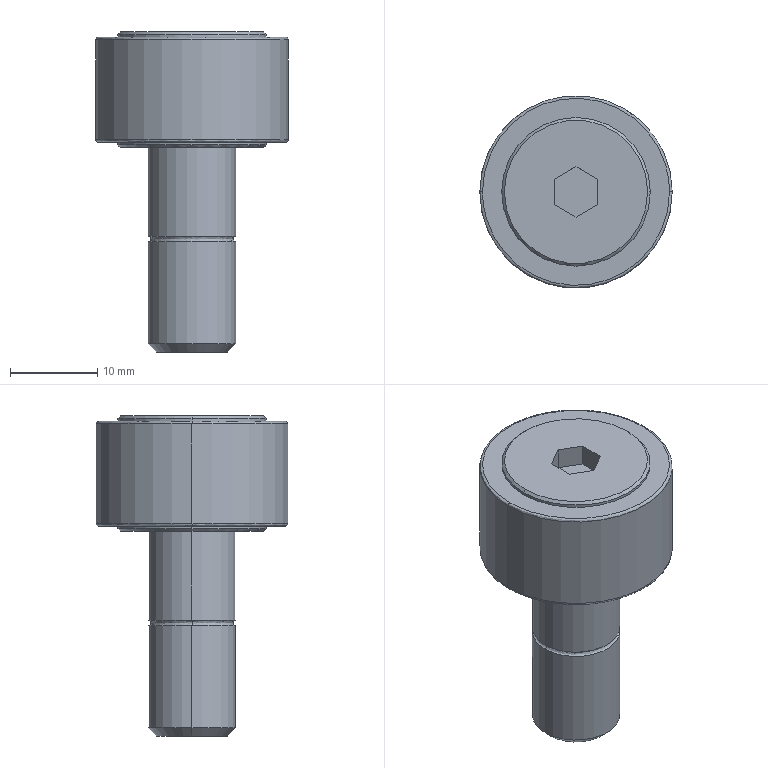Part | SolidWorks | features BaseBody 2 | 1 solid | 41 faces | box 22 x 22 x 36.6 mm | volume 6559 mm3 | plane 13 | cylinder 12 | cone 10 | spline 6 | commonest cylinder face diameters 10 x4 17 x4 3.242 x2 22 x2
STEP:
#1=CARTESIAN_POINT('',(11.,0.,-0.9));
#2=VERTEX_POINT('',#1);
#3=CARTESIAN_POINT('',(-11.,0.,-0.9));
#4=VERTEX_POINT('',#3);
#5=CARTESIAN_POINT('',(0.,0.,-0.9));
#6=DIRECTION('',(0.,0.,-1.));
#7=DIRECTION('',(1.,0.,0.));
#8=AXIS2_PLACEMENT_3D('',#5,#6,#7);
#9=CIRCLE('',#8,11.);
#10=EDGE_CURVE('',#2,#4,#9,.T.);
#11=ORIENTED_EDGE('',*,*,#10,.F.);
#12=CARTESIAN_POINT('',(10.7,0.,-0.6));
#13=VERTEX_POINT('',#12);
#14=CARTESIAN_POINT('',(10.7,0.,-0.9));
#15=DIRECTION('',(0.,-1.,0.));
#16=DIRECTION('',(1.,0.,0.));
#17=AXIS2_PLACEMENT_3D('',#14,#15,#16);
#18=CIRCLE('',#17,0.3);
#19=EDGE_CURVE('',#2,#13,#18,.T.);
#20=ORIENTED_EDGE('',*,*,#19,.T.);
#21=CARTESIAN_POINT('',(-10.7,0.,-0.6));
#22=VERTEX_POINT('',#21);
#23=CARTESIAN_POINT('',(10.7,0.,-0.6));
#24=CARTESIAN_POINT('',(10.7,-21.4,-0.6));
#25=CARTESIAN_POINT('',(-10.7,-21.4,-0.6));
#26=CARTESIAN_POINT('',(-10.7,0.,-0.6));
#27=(BOUNDED_CURVE()B_SPLINE_CURVE(3,(#23,#24,#25,#26),.UNSPECIFIED.,.F.,.T.)B_SPLINE_CURVE_WITH_KNOTS((4,4),(0.5,1.),.UNSPECIFIED.)CURVE()GEOMETRIC_REPRESENTATION_ITEM()RATIONAL_B_SPLINE_CURVE((1.,0.3333,0.3333,1.))REPRESENTATION_ITEM(''));
#28=EDGE_CURVE('',#13,#22,#27,.T.);
#29=ORIENTED_EDGE('',*,*,#28,.T.);
#30=CARTESIAN_POINT('',(-10.7,0.,-0.9));
#31=DIRECTION('',(0.,1.,0.));
#32=DIRECTION('',(-1.,0.,0.));
#33=AXIS2_PLACEMENT_3D('',#30,#31,#32);
#34=CIRCLE('',#33,0.3);
#35=EDGE_CURVE('',#4,#22,#34,.T.);
#36=ORIENTED_EDGE('',*,*,#35,.F.);
#37=EDGE_LOOP('',(#11,#20,#29,#36));
#38=FACE_OUTER_BOUND('',#37,.T.);
#39=CARTESIAN_POINT('',(11.,0.,-0.9));
#40=CARTESIAN_POINT('',(11.,-22.,-0.9));
#41=CARTESIAN_POINT('',(-11.,-22.,-0.9));
#42=CARTESIAN_POINT('',(-11.,0.,-0.9));
#43=CARTESIAN_POINT('',(11.,0.,-0.7243));
#44=CARTESIAN_POINT('',(11.,-22.,-0.7243));
#45=CARTESIAN_POINT('',(-11.,-22.,-0.7243));
#46=CARTESIAN_POINT('',(-11.,0.,-0.7243));
#47=CARTESIAN_POINT('',(10.876,0.,-0.6));
#48=CARTESIAN_POINT('',(10.876,-21.751,-0.6));
#49=CARTESIAN_POINT('',(-10.876,-21.751,-0.6));
#50=CARTESIAN_POINT('',(-10.876,0.,-0.6));
#51=CARTESIAN_POINT('',(10.7,0.,-0.6));
#52=CARTESIAN_POINT('',(10.7,-21.4,-0.6));
#53=CARTESIAN_POINT('',(-10.7,-21.4,-0.6));
#54=CARTESIAN_POINT('',(-10.7,0.,-0.6));
#55=(BOUNDED_SURFACE()B_SPLINE_SURFACE(3,3,((#39,#40,#41,#42),(#43,#44,#45,#46),(#47,#48,#49,#50),(#51,#52,#53,#54)),.UNSPECIFIED.,.F.,.F.,.T.)B_SPLINE_SURFACE_WITH_KNOTS((4,4),(4,4),(0.,1.),(0.,1.),.UNSPECIFIED.)GEOMETRIC_REPRESENTATION_ITEM()RATIONAL_B_SPLINE_SURFACE(((1.,0.3333,0.3333,1.),(0.8047,0.2682,0.2682,0.8047),(0.8047,0.2682,0.2682,0.8047),(1.,0.3333,0.3333,1.)))REPRESENTATION_ITEM('')SURFACE());
#56=ADVANCED_FACE('',(#38),#55,.T.);
#57=CARTESIAN_POINT('',(-10.7,0.,-12.6));
#58=VERTEX_POINT('',#57);
#59=CARTESIAN_POINT('',(10.7,0.,-12.6));
#60=VERTEX_POINT('',#59);
#61=CARTESIAN_POINT('',(-10.7,0.,-12.6));
#62=CARTESIAN_POINT('',(-10.7,-21.4,-12.6));
#63=CARTESIAN_POINT('',(10.7,-21.4,-12.6));
#64=CARTESIAN_POINT('',(10.7,0.,-12.6));
#65=(BOUNDED_CURVE()B_SPLINE_CURVE(3,(#61,#62,#63,#64),.UNSPECIFIED.,.F.,.T.)B_SPLINE_CURVE_WITH_KNOTS((4,4),(0.,0.5),.UNSPECIFIED.)CURVE()GEOMETRIC_REPRESENTATION_ITEM()RATIONAL_B_SPLINE_CURVE((1.,0.3333,0.3333,1.))REPRESENTATION_ITEM(''));
#66=EDGE_CURVE('',#58,#60,#65,.T.);
#67=ORIENTED_EDGE('',*,*,#66,.T.);
#68=CARTESIAN_POINT('',(11.,0.,-12.3));
#69=VERTEX_POINT('',#68);
#70=CARTESIAN_POINT('',(10.7,0.,-12.3));
#71=DIRECTION('',(0.,-1.,0.));
#72=DIRECTION('',(1.,0.,0.));
#73=AXIS2_PLACEMENT_3D('',#70,#71,#72);
#74=CIRCLE('',#73,0.3);
#75=EDGE_CURVE('',#60,#69,#74,.T.);
#76=ORIENTED_EDGE('',*,*,#75,.T.);
#77=CARTESIAN_POINT('',(-11.,0.,-12.3));
#78=VERTEX_POINT('',#77);
#79=CARTESIAN_POINT('',(0.,0.,-12.3));
#80=DIRECTION('',(0.,0.,1.));
#81=DIRECTION('',(1.,0.,0.));
#82=AXIS2_PLACEMENT_3D('',#79,#80,#81);
#83=CIRCLE('',#82,11.);
#84=EDGE_CURVE('',#78,#69,#83,.T.);
#85=ORIENTED_EDGE('',*,*,#84,.F.);
#86=CARTESIAN_POINT('',(-10.7,0.,-12.3));
#87=DIRECTION('',(0.,1.,0.));
#88=DIRECTION('',(-1.,0.,0.));
#89=AXIS2_PLACEMENT_3D('',#86,#87,#88);
#90=CIRCLE('',#89,0.3);
#91=EDGE_CURVE('',#58,#78,#90,.T.);
#92=ORIENTED_EDGE('',*,*,#91,.F.);
#93=EDGE_LOOP('',(#67,#76,#85,#92));
#94=FACE_OUTER_BOUND('',#93,.T.);
#95=CARTESIAN_POINT('',(10.7,0.,-12.6));
#96=CARTESIAN_POINT('',(10.7,-21.4,-12.6));
#97=CARTESIAN_POINT('',(-10.7,-21.4,-12.6));
#98=CARTESIAN_POINT('',(-10.7,0.,-12.6));
#99=CARTESIAN_POINT('',(10.876,0.,-12.6));
#100=CARTESIAN_POINT('',(10.876,-21.751,-12.6));
#101=CARTESIAN_POINT('',(-10.876,-21.751,-12.6));
#102=CARTESIAN_POINT('',(-10.876,0.,-12.6));
#103=CARTESIAN_POINT('',(11.,0.,-12.476));
#104=CARTESIAN_POINT('',(11.,-22.,-12.476));
#105=CARTESIAN_POINT('',(-11.,-22.,-12.476));
#106=CARTESIAN_POINT('',(-11.,0.,-12.476));
#107=CARTESIAN_POINT('',(11.,0.,-12.3));
#108=CARTESIAN_POINT('',(11.,-22.,-12.3));
#109=CARTESIAN_POINT('',(-11.,-22.,-12.3));
#110=CARTESIAN_POINT('',(-11.,0.,-12.3));
#111=(BOUNDED_SURFACE()B_SPLINE_SURFACE(3,3,((#95,#96,#97,#98),(#99,#100,#101,#102),(#103,#104,#105,#106),(#107,#108,#109,#110)),.UNSPECIFIED.,.F.,.F.,.F.)B_SPLINE_SURFACE_WITH_KNOTS((4,4),(4,4),(0.,1.),(0.,1.),.UNSPECIFIED.)GEOMETRIC_REPRESENTATION_ITEM()RATIONAL_B_SPLINE_SURFACE(((1.,0.3333,0.3333,1.),(0.8047,0.2682,0.2682,0.8047),(0.8047,0.2682,0.2682,0.8047),(1.,0.3333,0.3333,1.)))REPRESENTATION_ITEM('')SURFACE());
#112=ADVANCED_FACE('',(#94),#111,.T.);
#113=CARTESIAN_POINT('',(5.,0.,-23.375));
#114=VERTEX_POINT('',#113);
#115=CARTESIAN_POINT('',(-5.,0.,-23.375));
#116=VERTEX_POINT('',#115);
#117=CARTESIAN_POINT('',(0.,0.,-23.375));
#118=DIRECTION('',(0.,0.,1.));
#119=DIRECTION('',(1.,0.,0.));
#120=AXIS2_PLACEMENT_3D('',#117,#118,#119);
#121=CIRCLE('',#120,5.);
#122=EDGE_CURVE('',#114,#116,#121,.T.);
#123=ORIENTED_EDGE('',*,*,#122,.F.);
#124=CARTESIAN_POINT('',(5.,0.,-23.975));
#125=VERTEX_POINT('',#124);
#126=CARTESIAN_POINT('',(5.,0.,-23.675));
#127=DIRECTION('',(0.,-1.,0.));
#128=DIRECTION('',(1.,0.,0.));
#129=AXIS2_PLACEMENT_3D('',#126,#127,#128);
#130=CIRCLE('',#129,0.3);
#131=EDGE_CURVE('',#114,#125,#130,.T.);
#132=ORIENTED_EDGE('',*,*,#131,.T.);
#133=CARTESIAN_POINT('',(-5.,0.,-23.975));
#134=VERTEX_POINT('',#133);
#135=CARTESIAN_POINT('',(0.,0.,-23.975));
#136=DIRECTION('',(0.,0.,-1.));
#137=DIRECTION('',(-1.,0.,0.));
#138=AXIS2_PLACEMENT_3D('',#135,#136,#137);
#139=CIRCLE('',#138,5.);
#140=EDGE_CURVE('',#134,#125,#139,.T.);
#141=ORIENTED_EDGE('',*,*,#140,.F.);
#142=CARTESIAN_POINT('',(-5.,0.,-23.675));
#143=DIRECTION('',(0.,1.,0.));
#144=DIRECTION('',(-1.,0.,0.));
#145=AXIS2_PLACEMENT_3D('',#142,#143,#144);
#146=CIRCLE('',#145,0.3);
#147=EDGE_CURVE('',#116,#134,#146,.T.);
#148=ORIENTED_EDGE('',*,*,#147,.F.);
#149=EDGE_LOOP('',(#123,#132,#141,#148));
#150=FACE_OUTER_BOUND('',#149,.T.);
#151=CARTESIAN_POINT('',(-5.,0.,-23.375));
#152=CARTESIAN_POINT('',(-5.,10.,-23.375));
#153=CARTESIAN_POINT('',(5.,10.,-23.375));
#154=CARTESIAN_POINT('',(5.,0.,-23.375));
#155=CARTESIAN_POINT('',(-4.4,0.,-23.375));
#156=CARTESIAN_POINT('',(-4.4,8.8,-23.375));
#157=CARTESIAN_POINT('',(4.4,8.8,-23.375));
#158=CARTESIAN_POINT('',(4.4,0.,-23.375));
#159=CARTESIAN_POINT('',(-4.4,0.,-23.975));
#160=CARTESIAN_POINT('',(-4.4,8.8,-23.975));
#161=CARTESIAN_POINT('',(4.4,8.8,-23.975));
#162=CARTESIAN_POINT('',(4.4,0.,-23.975));
#163=CARTESIAN_POINT('',(-5.,0.,-23.975));
#164=CARTESIAN_POINT('',(-5.,10.,-23.975));
#165=CARTESIAN_POINT('',(5.,10.,-23.975));
#166=CARTESIAN_POINT('',(5.,0.,-23.975));
#167=(BOUNDED_SURFACE()B_SPLINE_SURFACE(3,3,((#151,#152,#153,#154),(#155,#156,#157,#158),(#159,#160,#161,#162),(#163,#164,#165,#166)),.UNSPECIFIED.,.F.,.F.,.F.)B_SPLINE_SURFACE_WITH_KNOTS((4,4),(4,4),(0.,1.),(0.,1.),.UNSPECIFIED.)GEOMETRIC_REPRESENTATION_ITEM()RATIONAL_B_SPLINE_SURFACE(((1.,0.3333,0.3333,1.),(0.3333,0.1111,0.1111,0.3333),(0.3333,0.1111,0.1111,0.3333),(1.,0.3333,0.3333,1.)))REPRESENTATION_ITEM('')SURFACE());
#168=ADVANCED_FACE('',(#150),#167,.F.);
#169=CARTESIAN_POINT('',(0.,0.,-12.3));
#170=DIRECTION('',(0.,0.,1.));
#171=DIRECTION('',(1.,0.,0.));
#172=AXIS2_PLACEMENT_3D('',#169,#170,#171);
#173=CIRCLE('',#172,11.);
#174=EDGE_CURVE('',#69,#78,#173,.T.);
#175=ORIENTED_EDGE('',*,*,#174,.T.);
#176=CARTESIAN_POINT('',(-11.,0.,-36.6));
#177=DIRECTION('',(0.,0.,1.));
#178=VECTOR('',#177,1000.);
#179=LINE('',#176,#178);
#180=EDGE_CURVE('',#78,#4,#179,.T.);
#181=ORIENTED_EDGE('',*,*,#180,.T.);
#182=CARTESIAN_POINT('',(0.,0.,-0.9));
#183=DIRECTION('',(0.,0.,-1.));
#184=DIRECTION('',(1.,0.,0.));
#185=AXIS2_PLACEMENT_3D('',#182,#183,#184);
#186=CIRCLE('',#185,11.);
#187=EDGE_CURVE('',#4,#2,#186,.T.);
#188=ORIENTED_EDGE('',*,*,#187,.T.);
#189=CARTESIAN_POINT('',(11.,0.,-36.6));
#190=DIRECTION('',(0.,0.,1.));
#191=VECTOR('',#190,1000.);
#192=LINE('',#189,#191);
#193=EDGE_CURVE('',#69,#2,#192,.T.);
#194=ORIENTED_EDGE('',*,*,#193,.F.);
#195=EDGE_LOOP('',(#175,#181,#188,#194));
#196=FACE_OUTER_BOUND('',#195,.T.);
#197=CARTESIAN_POINT('',(0.,0.,-36.6));
#198=DIRECTION('',(0.,0.,1.));
#199=DIRECTION('',(1.,0.,0.));
#200=AXIS2_PLACEMENT_3D('',#197,#198,#199);
#201=CYLINDRICAL_SURFACE('',#200,11.);
#202=ADVANCED_FACE('',(#196),#201,.T.);
#203=CARTESIAN_POINT('',(8.5,0.,-0.6));
#204=VERTEX_POINT('',#203);
#205=CARTESIAN_POINT('',(-8.5,0.,-0.6));
#206=VERTEX_POINT('',#205);
#207=CARTESIAN_POINT('',(0.,0.,-0.6));
#208=DIRECTION('',(0.,0.,1.));
#209=DIRECTION('',(1.,0.,0.));
#210=AXIS2_PLACEMENT_3D('',#207,#208,#209);
#211=CIRCLE('',#210,8.5);
#212=EDGE_CURVE('',#204,#206,#211,.T.);
#213=ORIENTED_EDGE('',*,*,#212,.T.);
#214=CARTESIAN_POINT('',(-8.5,0.,-0.3));
#215=VERTEX_POINT('',#214);
#216=CARTESIAN_POINT('',(-8.5,0.,-36.6));
#217=DIRECTION('',(0.,0.,1.));
#218=VECTOR('',#217,1000.);
#219=LINE('',#216,#218);
#220=EDGE_CURVE('',#206,#215,#219,.T.);
#221=ORIENTED_EDGE('',*,*,#220,.T.);
#222=CARTESIAN_POINT('',(8.5,0.,-0.3));
#223=VERTEX_POINT('',#222);
#224=CARTESIAN_POINT('',(0.,0.,-0.3));
#225=DIRECTION('',(0.,0.,-1.));
#226=DIRECTION('',(1.,0.,0.));
#227=AXIS2_PLACEMENT_3D('',#224,#225,#226);
#228=CIRCLE('',#227,8.5);
#229=EDGE_CURVE('',#215,#223,#228,.T.);
#230=ORIENTED_EDGE('',*,*,#229,.T.);
#231=CARTESIAN_POINT('',(8.5,0.,-36.6));
#232=DIRECTION('',(0.,0.,1.));
#233=VECTOR('',#232,1000.);
#234=LINE('',#231,#233);
#235=EDGE_CURVE('',#204,#223,#234,.T.);
#236=ORIENTED_EDGE('',*,*,#235,.F.);
#237=EDGE_LOOP('',(#213,#221,#230,#236));
#238=FACE_OUTER_BOUND('',#237,.T.);
#239=CARTESIAN_POINT('',(0.,0.,-36.6));
#240=DIRECTION('',(0.,0.,1.));
#241=DIRECTION('',(1.,0.,0.));
#242=AXIS2_PLACEMENT_3D('',#239,#240,#241);
#243=CYLINDRICAL_SURFACE('',#242,8.5);
#244=ADVANCED_FACE('',(#238),#243,.T.);
#245=CARTESIAN_POINT('',(8.5,0.,-12.9));
#246=VERTEX_POINT('',#245);
#247=CARTESIAN_POINT('',(-8.5,0.,-12.9));
#248=VERTEX_POINT('',#247);
#249=CARTESIAN_POINT('',(0.,0.,-12.9));
#250=DIRECTION('',(0.,0.,1.));
#251=DIRECTION('',(1.,0.,0.));
#252=AXIS2_PLACEMENT_3D('',#249,#250,#251);
#253=CIRCLE('',#252,8.5);
#254=EDGE_CURVE('',#246,#248,#253,.T.);
#255=ORIENTED_EDGE('',*,*,#254,.T.);
#256=CARTESIAN_POINT('',(-8.5,0.,-12.6));
#257=VERTEX_POINT('',#256);
#258=CARTESIAN_POINT('',(-8.5,0.,-36.6));
#259=DIRECTION('',(0.,0.,1.));
#260=VECTOR('',#259,1000.);
#261=LINE('',#258,#260);
#262=EDGE_CURVE('',#248,#257,#261,.T.);
#263=ORIENTED_EDGE('',*,*,#262,.T.);
#264=CARTESIAN_POINT('',(8.5,0.,-12.6));
#265=VERTEX_POINT('',#264);
#266=CARTESIAN_POINT('',(0.,0.,-12.6));
#267=DIRECTION('',(0.,0.,-1.));
#268=DIRECTION('',(1.,0.,0.));
#269=AXIS2_PLACEMENT_3D('',#266,#267,#268);
#270=CIRCLE('',#269,8.5);
#271=EDGE_CURVE('',#257,#265,#270,.T.);
#272=ORIENTED_EDGE('',*,*,#271,.T.);
#273=CARTESIAN_POINT('',(8.5,0.,-36.6));
#274=DIRECTION('',(0.,0.,1.));
#275=VECTOR('',#274,1000.);
#276=LINE('',#273,#275);
#277=EDGE_CURVE('',#246,#265,#276,.T.);
#278=ORIENTED_EDGE('',*,*,#277,.F.);
#279=EDGE_LOOP('',(#255,#263,#272,#278));
#280=FACE_OUTER_BOUND('',#279,.T.);
#281=CARTESIAN_POINT('',(0.,0.,-36.6));
#282=DIRECTION('',(0.,0.,1.));
#283=DIRECTION('',(1.,0.,0.));
#284=AXIS2_PLACEMENT_3D('',#281,#282,#283);
#285=CYLINDRICAL_SURFACE('',#284,8.5);
#286=ADVANCED_FACE('',(#280),#285,.T.);
#287=CARTESIAN_POINT('',(-8.2,0.,0.));
#288=VERTEX_POINT('',#287);
#289=CARTESIAN_POINT('',(8.2,0.,0.));
#290=VERTEX_POINT('',#289);
#291=CARTESIAN_POINT('',(0.,0.,0.));
#292=DIRECTION('',(0.,0.,-1.));
#293=DIRECTION('',(-1.,0.,0.));
#294=AXIS2_PLACEMENT_3D('',#291,#292,#293);
#295=CIRCLE('',#294,8.2);
#296=EDGE_CURVE('',#288,#290,#295,.T.);
#297=ORIENTED_EDGE('',*,*,#296,.T.);
#298=CARTESIAN_POINT('',(8.5,0.,-0.3));
#299=DIRECTION('',(0.7071,0.,-0.7071));
#300=VECTOR('',#299,1000.);
#301=LINE('',#298,#300);
#302=EDGE_CURVE('',#290,#223,#301,.T.);
#303=ORIENTED_EDGE('',*,*,#302,.T.);
#304=ORIENTED_EDGE('',*,*,#229,.F.);
#305=CARTESIAN_POINT('',(-8.5,0.,-0.3));
#306=DIRECTION('',(-0.7071,0.,-0.7071));
#307=VECTOR('',#306,1000.);
#308=LINE('',#305,#307);
#309=EDGE_CURVE('',#288,#215,#308,.T.);
#310=ORIENTED_EDGE('',*,*,#309,.F.);
#311=EDGE_LOOP('',(#297,#303,#304,#310));
#312=FACE_OUTER_BOUND('',#311,.T.);
#313=CARTESIAN_POINT('',(0.,0.,-0.3));
#314=DIRECTION('',(0.,0.,-1.));
#315=DIRECTION('',(-1.,0.,0.));
#316=AXIS2_PLACEMENT_3D('',#313,#314,#315);
#317=CONICAL_SURFACE('',#316,8.5,0.7854);
#318=ADVANCED_FACE('',(#312),#317,.T.);
#319=CARTESIAN_POINT('',(8.2,0.,-13.2));
#320=VERTEX_POINT('',#319);
#321=CARTESIAN_POINT('',(-8.2,0.,-13.2));
#322=VERTEX_POINT('',#321);
#323=CARTESIAN_POINT('',(0.,0.,-13.2));
#324=DIRECTION('',(0.,0.,1.));
#325=DIRECTION('',(1.,0.,0.));
#326=AXIS2_PLACEMENT_3D('',#323,#324,#325);
#327=CIRCLE('',#326,8.2);
#328=EDGE_CURVE('',#320,#322,#327,.T.);
#329=ORIENTED_EDGE('',*,*,#328,.T.);
#330=CARTESIAN_POINT('',(-8.5,0.,-12.9));
#331=DIRECTION('',(-0.7071,0.,0.7071));
#332=VECTOR('',#331,1000.);
#333=LINE('',#330,#332);
#334=EDGE_CURVE('',#322,#248,#333,.T.);
#335=ORIENTED_EDGE('',*,*,#334,.T.);
#336=ORIENTED_EDGE('',*,*,#254,.F.);
#337=CARTESIAN_POINT('',(8.5,0.,-12.9));
#338=DIRECTION('',(0.7071,0.,0.7071));
#339=VECTOR('',#338,1000.);
#340=LINE('',#337,#339);
#341=EDGE_CURVE('',#320,#246,#340,.T.);
#342=ORIENTED_EDGE('',*,*,#341,.F.);
#343=EDGE_LOOP('',(#329,#335,#336,#342));
#344=FACE_OUTER_BOUND('',#343,.T.);
#345=CARTESIAN_POINT('',(0.,0.,-12.9));
#346=DIRECTION('',(0.,0.,1.));
#347=DIRECTION('',(1.,0.,0.));
#348=AXIS2_PLACEMENT_3D('',#345,#346,#347);
#349=CONICAL_SURFACE('',#348,8.5,0.7854);
#350=ADVANCED_FACE('',(#344),#349,.T.);
#351=ORIENTED_EDGE('',*,*,#122,.T.);
#352=CARTESIAN_POINT('',(-5.,0.,-13.2));
#353=VERTEX_POINT('',#352);
#354=CARTESIAN_POINT('',(-5.,0.,-36.6));
#355=DIRECTION('',(0.,0.,1.));
#356=VECTOR('',#355,1000.);
#357=LINE('',#354,#356);
#358=EDGE_CURVE('',#116,#353,#357,.T.);
#359=ORIENTED_EDGE('',*,*,#358,.T.);
#360=CARTESIAN_POINT('',(5.,0.,-13.2));
#361=VERTEX_POINT('',#360);
#362=CARTESIAN_POINT('',(0.,0.,-13.2));
#363=DIRECTION('',(0.,0.,-1.));
#364=DIRECTION('',(1.,0.,0.));
#365=AXIS2_PLACEMENT_3D('',#362,#363,#364);
#366=CIRCLE('',#365,5.);
#367=EDGE_CURVE('',#353,#361,#366,.T.);
#368=ORIENTED_EDGE('',*,*,#367,.T.);
#369=CARTESIAN_POINT('',(5.,0.,-36.6));
#370=DIRECTION('',(0.,0.,1.));
#371=VECTOR('',#370,1000.);
#372=LINE('',#369,#371);
#373=EDGE_CURVE('',#114,#361,#372,.T.);
#374=ORIENTED_EDGE('',*,*,#373,.F.);
#375=EDGE_LOOP('',(#351,#359,#368,#374));
#376=FACE_OUTER_BOUND('',#375,.T.);
#377=CARTESIAN_POINT('',(0.,0.,-36.6));
#378=DIRECTION('',(0.,0.,1.));
#379=DIRECTION('',(1.,0.,0.));
#380=AXIS2_PLACEMENT_3D('',#377,#378,#379);
#381=CYLINDRICAL_SURFACE('',#380,5.);
#382=ADVANCED_FACE('',(#376),#381,.T.);
#383=CARTESIAN_POINT('',(5.,0.,-35.68));
#384=VERTEX_POINT('',#383);
#385=CARTESIAN_POINT('',(-5.,0.,-35.68));
#386=VERTEX_POINT('',#385);
#387=CARTESIAN_POINT('',(0.,0.,-35.68));
#388=DIRECTION('',(0.,0.,1.));
#389=DIRECTION('',(1.,0.,0.));
#390=AXIS2_PLACEMENT_3D('',#387,#388,#389);
#391=CIRCLE('',#390,5.);
#392=EDGE_CURVE('',#384,#386,#391,.T.);
#393=ORIENTED_EDGE('',*,*,#392,.T.);
#394=CARTESIAN_POINT('',(-5.,0.,-36.6));
#395=DIRECTION('',(0.,0.,1.));
#396=VECTOR('',#395,1000.);
#397=LINE('',#394,#396);
#398=EDGE_CURVE('',#386,#134,#397,.T.);
#399=ORIENTED_EDGE('',*,*,#398,.T.);
#400=ORIENTED_EDGE('',*,*,#140,.T.);
#401=CARTESIAN_POINT('',(5.,0.,-36.6));
#402=DIRECTION('',(0.,0.,1.));
#403=VECTOR('',#402,1000.);
#404=LINE('',#401,#403);
#405=EDGE_CURVE('',#384,#125,#404,.T.);
#406=ORIENTED_EDGE('',*,*,#405,.F.);
#407=EDGE_LOOP('',(#393,#399,#400,#406));
#408=FACE_OUTER_BOUND('',#407,.T.);
#409=CARTESIAN_POINT('',(0.,0.,-36.6));
#410=DIRECTION('',(0.,0.,1.));
#411=DIRECTION('',(1.,0.,0.));
#412=AXIS2_PLACEMENT_3D('',#409,#410,#411);
#413=CYLINDRICAL_SURFACE('',#412,5.);
#414=ADVANCED_FACE('',(#408),#413,.T.);
#415=CARTESIAN_POINT('',(4.08,0.,-36.6));
#416=VERTEX_POINT('',#415);
#417=CARTESIAN_POINT('',(-4.08,0.,-36.6));
#418=VERTEX_POINT('',#417);
#419=CARTESIAN_POINT('',(0.,0.,-36.6));
#420=DIRECTION('',(0.,0.,1.));
#421=DIRECTION('',(1.,0.,0.));
#422=AXIS2_PLACEMENT_3D('',#419,#420,#421);
#423=CIRCLE('',#422,4.08);
#424=EDGE_CURVE('',#416,#418,#423,.T.);
#425=ORIENTED_EDGE('',*,*,#424,.T.);
#426=CARTESIAN_POINT('',(-5.,0.,-35.68));
#427=DIRECTION('',(-0.7071,0.,0.7071));
#428=VECTOR('',#427,1000.);
#429=LINE('',#426,#428);
#430=EDGE_CURVE('',#418,#386,#429,.T.);
#431=ORIENTED_EDGE('',*,*,#430,.T.);
#432=ORIENTED_EDGE('',*,*,#392,.F.);
#433=CARTESIAN_POINT('',(5.,0.,-35.68));
#434=DIRECTION('',(0.7071,0.,0.7071));
#435=VECTOR('',#434,1000.);
#436=LINE('',#433,#435);
#437=EDGE_CURVE('',#416,#384,#436,.T.);
#438=ORIENTED_EDGE('',*,*,#437,.F.);
#439=EDGE_LOOP('',(#425,#431,#432,#438));
#440=FACE_OUTER_BOUND('',#439,.T.);
#441=CARTESIAN_POINT('',(0.,0.,-35.68));
#442=DIRECTION('',(0.,0.,1.));
#443=DIRECTION('',(1.,0.,0.));
#444=AXIS2_PLACEMENT_3D('',#441,#442,#443);
#445=CONICAL_SURFACE('',#444,5.,0.7854);
#446=ADVANCED_FACE('',(#440),#445,.T.);
#447=CARTESIAN_POINT('',(1.621,0.,-36.221));
#448=VERTEX_POINT('',#447);
#449=CARTESIAN_POINT('',(-1.621,0.,-36.221));
#450=VERTEX_POINT('',#449);
#451=CARTESIAN_POINT('',(0.,0.,-36.221));
#452=DIRECTION('',(0.,0.,-1.));
#453=DIRECTION('',(-1.,0.,0.));
#454=AXIS2_PLACEMENT_3D('',#451,#452,#453);
#455=CIRCLE('',#454,1.621);
#456=EDGE_CURVE('',#448,#450,#455,.T.);
#457=ORIENTED_EDGE('',*,*,#456,.F.);
#458=CARTESIAN_POINT('',(2.,0.,-36.6));
#459=VERTEX_POINT('',#458);
#460=CARTESIAN_POINT('',(2.,0.,-36.6));
#461=DIRECTION('',(0.7071,0.,-0.7071));
#462=VECTOR('',#461,1000.);
#463=LINE('',#460,#462);
#464=EDGE_CURVE('',#448,#459,#463,.T.);
#465=ORIENTED_EDGE('',*,*,#464,.T.);
#466=CARTESIAN_POINT('',(-2.,0.,-36.6));
#467=VERTEX_POINT('',#466);
#468=CARTESIAN_POINT('',(0.,0.,-36.6));
#469=DIRECTION('',(0.,0.,-1.));
#470=DIRECTION('',(-1.,0.,0.));
#471=AXIS2_PLACEMENT_3D('',#468,#469,#470);
#472=CIRCLE('',#471,2.);
#473=EDGE_CURVE('',#459,#467,#472,.T.);
#474=ORIENTED_EDGE('',*,*,#473,.T.);
#475=CARTESIAN_POINT('',(-2.,0.,-36.6));
#476=DIRECTION('',(-0.7071,0.,-0.7071));
#477=VECTOR('',#476,1000.);
#478=LINE('',#475,#477);
#479=EDGE_CURVE('',#450,#467,#478,.T.);
#480=ORIENTED_EDGE('',*,*,#479,.F.);
#481=EDGE_LOOP('',(#457,#465,#474,#480));
#482=FACE_OUTER_BOUND('',#481,.T.);
#483=CARTESIAN_POINT('',(0.,0.,-36.6));
#484=DIRECTION('',(0.,0.,-1.));
#485=DIRECTION('',(-1.,0.,0.));
#486=AXIS2_PLACEMENT_3D('',#483,#484,#485);
#487=CONICAL_SURFACE('',#486,2.,0.7854);
#488=ADVANCED_FACE('',(#482),#487,.F.);
#489=ORIENTED_EDGE('',*,*,#456,.T.);
#490=CARTESIAN_POINT('',(-1.621,0.,-32.979));
#491=VERTEX_POINT('',#490);
#492=CARTESIAN_POINT('',(-1.621,0.,-36.6));
#493=DIRECTION('',(0.,0.,1.));
#494=VECTOR('',#493,1000.);
#495=LINE('',#492,#494);
#496=EDGE_CURVE('',#450,#491,#495,.T.);
#497=ORIENTED_EDGE('',*,*,#496,.T.);
#498=CARTESIAN_POINT('',(1.621,0.,-32.979));
#499=VERTEX_POINT('',#498);
#500=CARTESIAN_POINT('',(0.,0.,-32.979));
#501=DIRECTION('',(0.,0.,-1.));
#502=DIRECTION('',(1.,0.,0.));
#503=AXIS2_PLACEMENT_3D('',#500,#501,#502);
#504=CIRCLE('',#503,1.621);
#505=EDGE_CURVE('',#499,#491,#504,.T.);
#506=ORIENTED_EDGE('',*,*,#505,.F.);
#507=CARTESIAN_POINT('',(1.621,0.,-36.6));
#508=DIRECTION('',(0.,0.,1.));
#509=VECTOR('',#508,1000.);
#510=LINE('',#507,#509);
#511=EDGE_CURVE('',#448,#499,#510,.T.);
#512=ORIENTED_EDGE('',*,*,#511,.F.);
#513=EDGE_LOOP('',(#489,#497,#506,#512));
#514=FACE_OUTER_BOUND('',#513,.T.);
#515=CARTESIAN_POINT('',(0.,0.,-36.6));
#516=DIRECTION('',(0.,0.,1.));
#517=DIRECTION('',(1.,0.,0.));
#518=AXIS2_PLACEMENT_3D('',#515,#516,#517);
#519=CYLINDRICAL_SURFACE('',#518,1.621);
#520=ADVANCED_FACE('',(#514),#519,.F.);
#521=ORIENTED_EDGE('',*,*,#505,.T.);
#522=CARTESIAN_POINT('',(-2.,0.,-32.6));
#523=VERTEX_POINT('',#522);
#524=CARTESIAN_POINT('',(-2.,0.,-32.6));
#525=DIRECTION('',(-0.7071,0.,0.7071));
#526=VECTOR('',#525,1000.);
#527=LINE('',#524,#526);
#528=EDGE_CURVE('',#491,#523,#527,.T.);
#529=ORIENTED_EDGE('',*,*,#528,.T.);
#530=CARTESIAN_POINT('',(2.,0.,-32.6));
#531=VERTEX_POINT('',#530);
#532=CARTESIAN_POINT('',(0.,0.,-32.6));
#533=DIRECTION('',(0.,0.,-1.));
#534=DIRECTION('',(1.,0.,0.));
#535=AXIS2_PLACEMENT_3D('',#532,#533,#534);
#536=CIRCLE('',#535,2.);
#537=EDGE_CURVE('',#531,#523,#536,.T.);
#538=ORIENTED_EDGE('',*,*,#537,.F.);
#539=CARTESIAN_POINT('',(2.,0.,-32.6));
#540=DIRECTION('',(0.7071,0.,0.7071));
#541=VECTOR('',#540,1000.);
#542=LINE('',#539,#541);
#543=EDGE_CURVE('',#499,#531,#542,.T.);
#544=ORIENTED_EDGE('',*,*,#543,.F.);
#545=EDGE_LOOP('',(#521,#529,#538,#544));
#546=FACE_OUTER_BOUND('',#545,.T.);
#547=CARTESIAN_POINT('',(0.,0.,-32.6));
#548=DIRECTION('',(0.,0.,1.));
#549=DIRECTION('',(1.,0.,0.));
#550=AXIS2_PLACEMENT_3D('',#547,#548,#549);
#551=CONICAL_SURFACE('',#550,2.,0.7854);
#552=ADVANCED_FACE('',(#546),#551,.F.);
#553=ORIENTED_EDGE('',*,*,#180,.F.);
#554=ORIENTED_EDGE('',*,*,#84,.T.);
#555=ORIENTED_EDGE('',*,*,#193,.T.);
#556=ORIENTED_EDGE('',*,*,#10,.T.);
#557=EDGE_LOOP('',(#553,#554,#555,#556));
#558=FACE_OUTER_BOUND('',#557,.T.);
#559=CARTESIAN_POINT('',(0.,0.,-36.6));
#560=DIRECTION('',(0.,0.,1.));
#561=DIRECTION('',(1.,0.,0.));
#562=AXIS2_PLACEMENT_3D('',#559,#560,#561);
#563=CYLINDRICAL_SURFACE('',#562,11.);
#564=ADVANCED_FACE('',(#558),#563,.T.);
#565=ORIENTED_EDGE('',*,*,#19,.F.);
#566=ORIENTED_EDGE('',*,*,#187,.F.);
#567=ORIENTED_EDGE('',*,*,#35,.T.);
#568=CARTESIAN_POINT('',(-10.7,0.,-0.6));
#569=CARTESIAN_POINT('',(-10.7,21.4,-0.6));
#570=CARTESIAN_POINT('',(10.7,21.4,-0.6));
#571=CARTESIAN_POINT('',(10.7,0.,-0.6));
#572=(BOUNDED_CURVE()B_SPLINE_CURVE(3,(#568,#569,#570,#571),.UNSPECIFIED.,.F.,.T.)B_SPLINE_CURVE_WITH_KNOTS((4,4),(0.,0.5),.UNSPECIFIED.)CURVE()GEOMETRIC_REPRESENTATION_ITEM()RATIONAL_B_SPLINE_CURVE((1.,0.3333,0.3333,1.))REPRESENTATION_ITEM(''));
#573=EDGE_CURVE('',#22,#13,#572,.T.);
#574=ORIENTED_EDGE('',*,*,#573,.T.);
#575=EDGE_LOOP('',(#565,#566,#567,#574));
#576=FACE_OUTER_BOUND('',#575,.T.);
#577=CARTESIAN_POINT('',(-11.,0.,-0.9));
#578=CARTESIAN_POINT('',(-11.,22.,-0.9));
#579=CARTESIAN_POINT('',(11.,22.,-0.9));
#580=CARTESIAN_POINT('',(11.,0.,-0.9));
#581=CARTESIAN_POINT('',(-11.,0.,-0.7243));
#582=CARTESIAN_POINT('',(-11.,22.,-0.7243));
#583=CARTESIAN_POINT('',(11.,22.,-0.7243));
#584=CARTESIAN_POINT('',(11.,0.,-0.7243));
#585=CARTESIAN_POINT('',(-10.876,0.,-0.6));
#586=CARTESIAN_POINT('',(-10.876,21.751,-0.6));
#587=CARTESIAN_POINT('',(10.876,21.751,-0.6));
#588=CARTESIAN_POINT('',(10.876,0.,-0.6));
#589=CARTESIAN_POINT('',(-10.7,0.,-0.6));
#590=CARTESIAN_POINT('',(-10.7,21.4,-0.6));
#591=CARTESIAN_POINT('',(10.7,21.4,-0.6));
#592=CARTESIAN_POINT('',(10.7,0.,-0.6));
#593=(BOUNDED_SURFACE()B_SPLINE_SURFACE(3,3,((#577,#578,#579,#580),(#581,#582,#583,#584),(#585,#586,#587,#588),(#589,#590,#591,#592)),.UNSPECIFIED.,.F.,.F.,.T.)B_SPLINE_SURFACE_WITH_KNOTS((4,4),(4,4),(0.,1.),(0.,1.),.UNSPECIFIED.)GEOMETRIC_REPRESENTATION_ITEM()RATIONAL_B_SPLINE_SURFACE(((1.,0.3333,0.3333,1.),(0.8047,0.2682,0.2682,0.8047),(0.8047,0.2682,0.2682,0.8047),(1.,0.3333,0.3333,1.)))REPRESENTATION_ITEM('')SURFACE());
#594=ADVANCED_FACE('',(#576),#593,.T.);
#595=ORIENTED_EDGE('',*,*,#75,.F.);
#596=CARTESIAN_POINT('',(10.7,0.,-12.6));
#597=CARTESIAN_POINT('',(10.7,21.4,-12.6));
#598=CARTESIAN_POINT('',(-10.7,21.4,-12.6));
#599=CARTESIAN_POINT('',(-10.7,0.,-12.6));
#600=(BOUNDED_CURVE()B_SPLINE_CURVE(3,(#596,#597,#598,#599),.UNSPECIFIED.,.F.,.T.)B_SPLINE_CURVE_WITH_KNOTS((4,4),(0.5,1.),.UNSPECIFIED.)CURVE()GEOMETRIC_REPRESENTATION_ITEM()RATIONAL_B_SPLINE_CURVE((1.,0.3333,0.3333,1.))REPRESENTATION_ITEM(''));
#601=EDGE_CURVE('',#60,#58,#600,.T.);
#602=ORIENTED_EDGE('',*,*,#601,.T.);
#603=ORIENTED_EDGE('',*,*,#91,.T.);
#604=ORIENTED_EDGE('',*,*,#174,.F.);
#605=EDGE_LOOP('',(#595,#602,#603,#604));
#606=FACE_OUTER_BOUND('',#605,.T.);
#607=CARTESIAN_POINT('',(-10.7,0.,-12.6));
#608=CARTESIAN_POINT('',(-10.7,21.4,-12.6));
#609=CARTESIAN_POINT('',(10.7,21.4,-12.6));
#610=CARTESIAN_POINT('',(10.7,0.,-12.6));
#611=CARTESIAN_POINT('',(-10.876,0.,-12.6));
#612=CARTESIAN_POINT('',(-10.876,21.751,-12.6));
#613=CARTESIAN_POINT('',(10.876,21.751,-12.6));
#614=CARTESIAN_POINT('',(10.876,0.,-12.6));
#615=CARTESIAN_POINT('',(-11.,0.,-12.476));
#616=CARTESIAN_POINT('',(-11.,22.,-12.476));
#617=CARTESIAN_POINT('',(11.,22.,-12.476));
#618=CARTESIAN_POINT('',(11.,0.,-12.476));
#619=CARTESIAN_POINT('',(-11.,0.,-12.3));
#620=CARTESIAN_POINT('',(-11.,22.,-12.3));
#621=CARTESIAN_POINT('',(11.,22.,-12.3));
#622=CARTESIAN_POINT('',(11.,0.,-12.3));
#623=(BOUNDED_SURFACE()B_SPLINE_SURFACE(3,3,((#607,#608,#609,#610),(#611,#612,#613,#614),(#615,#616,#617,#618),(#619,#620,#621,#622)),.UNSPECIFIED.,.F.,.F.,.T.)B_SPLINE_SURFACE_WITH_KNOTS((4,4),(4,4),(0.,1.),(0.,1.),.UNSPECIFIED.)GEOMETRIC_REPRESENTATION_ITEM()RATIONAL_B_SPLINE_SURFACE(((1.,0.3333,0.3333,1.),(0.8047,0.2682,0.2682,0.8047),(0.8047,0.2682,0.2682,0.8047),(1.,0.3333,0.3333,1.)))REPRESENTATION_ITEM('')SURFACE());
#624=ADVANCED_FACE('',(#606),#623,.T.);
#625=ORIENTED_EDGE('',*,*,#212,.F.);
#626=CARTESIAN_POINT('',(0.,0.,-0.6));
#627=DIRECTION('',(0.,0.,1.));
#628=DIRECTION('',(1.,0.,0.));
#629=AXIS2_PLACEMENT_3D('',#626,#627,#628);
#630=CIRCLE('',#629,8.5);
#631=EDGE_CURVE('',#206,#204,#630,.T.);
#632=ORIENTED_EDGE('',*,*,#631,.F.);
#633=EDGE_LOOP('',(#625,#632));
#634=FACE_BOUND('',#633,.T.);
#635=ORIENTED_EDGE('',*,*,#573,.F.);
#636=ORIENTED_EDGE('',*,*,#28,.F.);
#637=EDGE_LOOP('',(#635,#636));
#638=FACE_OUTER_BOUND('',#637,.T.);
#639=CARTESIAN_POINT('',(0.,8.5,-0.6));
#640=DIRECTION('',(0.,0.,-1.));
#641=DIRECTION('',(-1.,0.,0.));
#642=AXIS2_PLACEMENT_3D('',#639,#640,#641);
#643=PLANE('',#642);
#644=ADVANCED_FACE('',(#634,#638),#643,.F.);
#645=ORIENTED_EDGE('',*,*,#66,.F.);
#646=ORIENTED_EDGE('',*,*,#601,.F.);
#647=EDGE_LOOP('',(#645,#646));
#648=FACE_OUTER_BOUND('',#647,.T.);
#649=CARTESIAN_POINT('',(0.,0.,-12.6));
#650=DIRECTION('',(0.,0.,-1.));
#651=DIRECTION('',(1.,0.,0.));
#652=AXIS2_PLACEMENT_3D('',#649,#650,#651);
#653=CIRCLE('',#652,8.5);
#654=EDGE_CURVE('',#265,#257,#653,.T.);
#655=ORIENTED_EDGE('',*,*,#654,.F.);
#656=ORIENTED_EDGE('',*,*,#271,.F.);
#657=EDGE_LOOP('',(#655,#656));
#658=FACE_BOUND('',#657,.T.);
#659=CARTESIAN_POINT('',(0.,10.7,-12.6));
#660=DIRECTION('',(0.,0.,1.));
#661=DIRECTION('',(1.,0.,0.));
#662=AXIS2_PLACEMENT_3D('',#659,#660,#661);
#663=PLANE('',#662);
#664=ADVANCED_FACE('',(#648,#658),#663,.F.);
#665=ORIENTED_EDGE('',*,*,#220,.F.);
#666=ORIENTED_EDGE('',*,*,#631,.T.);
#667=ORIENTED_EDGE('',*,*,#235,.T.);
#668=CARTESIAN_POINT('',(0.,0.,-0.3));
#669=DIRECTION('',(0.,0.,-1.));
#670=DIRECTION('',(1.,0.,0.));
#671=AXIS2_PLACEMENT_3D('',#668,#669,#670);
#672=CIRCLE('',#671,8.5);
#673=EDGE_CURVE('',#223,#215,#672,.T.);
#674=ORIENTED_EDGE('',*,*,#673,.T.);
#675=EDGE_LOOP('',(#665,#666,#667,#674));
#676=FACE_OUTER_BOUND('',#675,.T.);
#677=CARTESIAN_POINT('',(0.,0.,-36.6));
#678=DIRECTION('',(0.,0.,1.));
#679=DIRECTION('',(1.,0.,0.));
#680=AXIS2_PLACEMENT_3D('',#677,#678,#679);
#681=CYLINDRICAL_SURFACE('',#680,8.5);
#682=ADVANCED_FACE('',(#676),#681,.T.);
#683=ORIENTED_EDGE('',*,*,#262,.F.);
#684=CARTESIAN_POINT('',(0.,0.,-12.9));
#685=DIRECTION('',(0.,0.,1.));
#686=DIRECTION('',(1.,0.,0.));
#687=AXIS2_PLACEMENT_3D('',#684,#685,#686);
#688=CIRCLE('',#687,8.5);
#689=EDGE_CURVE('',#248,#246,#688,.T.);
#690=ORIENTED_EDGE('',*,*,#689,.T.);
#691=ORIENTED_EDGE('',*,*,#277,.T.);
#692=ORIENTED_EDGE('',*,*,#654,.T.);
#693=EDGE_LOOP('',(#683,#690,#691,#692));
#694=FACE_OUTER_BOUND('',#693,.T.);
#695=CARTESIAN_POINT('',(0.,0.,-36.6));
#696=DIRECTION('',(0.,0.,1.));
#697=DIRECTION('',(1.,0.,0.));
#698=AXIS2_PLACEMENT_3D('',#695,#696,#697);
#699=CYLINDRICAL_SURFACE('',#698,8.5);
#700=ADVANCED_FACE('',(#694),#699,.T.);
#701=ORIENTED_EDGE('',*,*,#302,.F.);
#702=CARTESIAN_POINT('',(0.,0.,0.));
#703=DIRECTION('',(0.,0.,-1.));
#704=DIRECTION('',(-1.,0.,0.));
#705=AXIS2_PLACEMENT_3D('',#702,#703,#704);
#706=CIRCLE('',#705,8.2);
#707=EDGE_CURVE('',#290,#288,#706,.T.);
#708=ORIENTED_EDGE('',*,*,#707,.T.);
#709=ORIENTED_EDGE('',*,*,#309,.T.);
#710=ORIENTED_EDGE('',*,*,#673,.F.);
#711=EDGE_LOOP('',(#701,#708,#709,#710));
#712=FACE_OUTER_BOUND('',#711,.T.);
#713=CARTESIAN_POINT('',(0.,0.,-0.3));
#714=DIRECTION('',(0.,0.,-1.));
#715=DIRECTION('',(-1.,0.,0.));
#716=AXIS2_PLACEMENT_3D('',#713,#714,#715);
#717=CONICAL_SURFACE('',#716,8.5,0.7854);
#718=ADVANCED_FACE('',(#712),#717,.T.);
#719=ORIENTED_EDGE('',*,*,#334,.F.);
#720=CARTESIAN_POINT('',(0.,0.,-13.2));
#721=DIRECTION('',(0.,0.,1.));
#722=DIRECTION('',(1.,0.,0.));
#723=AXIS2_PLACEMENT_3D('',#720,#721,#722);
#724=CIRCLE('',#723,8.2);
#725=EDGE_CURVE('',#322,#320,#724,.T.);
#726=ORIENTED_EDGE('',*,*,#725,.T.);
#727=ORIENTED_EDGE('',*,*,#341,.T.);
#728=ORIENTED_EDGE('',*,*,#689,.F.);
#729=EDGE_LOOP('',(#719,#726,#727,#728));
#730=FACE_OUTER_BOUND('',#729,.T.);
#731=CARTESIAN_POINT('',(0.,0.,-12.9));
#732=DIRECTION('',(0.,0.,1.));
#733=DIRECTION('',(1.,0.,0.));
#734=AXIS2_PLACEMENT_3D('',#731,#732,#733);
#735=CONICAL_SURFACE('',#734,8.5,0.7854);
#736=ADVANCED_FACE('',(#730),#735,.T.);
#737=CARTESIAN_POINT('',(-2.5,1.443,0.));
#738=VERTEX_POINT('',#737);
#739=CARTESIAN_POINT('',(-2.5,-1.443,0.));
#740=VERTEX_POINT('',#739);
#741=CARTESIAN_POINT('',(-2.5,0.,0.));
#742=DIRECTION('',(0.,-1.,0.));
#743=VECTOR('',#742,1000.);
#744=LINE('',#741,#743);
#745=EDGE_CURVE('',#738,#740,#744,.T.);
#746=ORIENTED_EDGE('',*,*,#745,.F.);
#747=CARTESIAN_POINT('',(0.,2.887,0.));
#748=VERTEX_POINT('',#747);
#749=CARTESIAN_POINT('',(0.,2.887,0.));
#750=DIRECTION('',(-0.866,-0.5,0.));
#751=VECTOR('',#750,1000.);
#752=LINE('',#749,#751);
#753=EDGE_CURVE('',#748,#738,#752,.T.);
#754=ORIENTED_EDGE('',*,*,#753,.F.);
#755=CARTESIAN_POINT('',(2.5,1.443,0.));
#756=VERTEX_POINT('',#755);
#757=CARTESIAN_POINT('',(2.5,1.443,0.));
#758=DIRECTION('',(-0.866,0.5,0.));
#759=VECTOR('',#758,1000.);
#760=LINE('',#757,#759);
#761=EDGE_CURVE('',#756,#748,#760,.T.);
#762=ORIENTED_EDGE('',*,*,#761,.F.);
#763=CARTESIAN_POINT('',(2.5,-1.443,0.));
#764=VERTEX_POINT('',#763);
#765=CARTESIAN_POINT('',(2.5,0.,0.));
#766=DIRECTION('',(0.,1.,0.));
#767=VECTOR('',#766,1000.);
#768=LINE('',#765,#767);
#769=EDGE_CURVE('',#764,#756,#768,.T.);
#770=ORIENTED_EDGE('',*,*,#769,.F.);
#771=CARTESIAN_POINT('',(0.,-2.887,0.));
#772=VERTEX_POINT('',#771);
#773=CARTESIAN_POINT('',(0.,-2.887,0.));
#774=DIRECTION('',(0.866,0.5,0.));
#775=VECTOR('',#774,1000.);
#776=LINE('',#773,#775);
#777=EDGE_CURVE('',#772,#764,#776,.T.);
#778=ORIENTED_EDGE('',*,*,#777,.F.);
#779=CARTESIAN_POINT('',(-2.5,-1.443,0.));
#780=DIRECTION('',(0.866,-0.5,0.));
#781=VECTOR('',#780,1000.);
#782=LINE('',#779,#781);
#783=EDGE_CURVE('',#740,#772,#782,.T.);
#784=ORIENTED_EDGE('',*,*,#783,.F.);
#785=EDGE_LOOP('',(#746,#754,#762,#770,#778,#784));
#786=FACE_BOUND('',#785,.T.);
#787=ORIENTED_EDGE('',*,*,#296,.F.);
#788=ORIENTED_EDGE('',*,*,#707,.F.);
#789=EDGE_LOOP('',(#787,#788));
#790=FACE_OUTER_BOUND('',#789,.T.);
#791=CARTESIAN_POINT('',(0.,0.,0.));
#792=DIRECTION('',(0.,0.,-1.));
#793=DIRECTION('',(-1.,0.,0.));
#794=AXIS2_PLACEMENT_3D('',#791,#792,#793);
#795=PLANE('',#794);
#796=ADVANCED_FACE('',(#786,#790),#795,.F.);
#797=ORIENTED_EDGE('',*,*,#328,.F.);
#798=ORIENTED_EDGE('',*,*,#725,.F.);
#799=EDGE_LOOP('',(#797,#798));
#800=FACE_OUTER_BOUND('',#799,.T.);
#801=CARTESIAN_POINT('',(0.,0.,-13.2));
#802=DIRECTION('',(0.,0.,-1.));
#803=DIRECTION('',(1.,0.,0.));
#804=AXIS2_PLACEMENT_3D('',#801,#802,#803);
#805=CIRCLE('',#804,5.);
#806=EDGE_CURVE('',#361,#353,#805,.T.);
#807=ORIENTED_EDGE('',*,*,#806,.F.);
#808=ORIENTED_EDGE('',*,*,#367,.F.);
#809=EDGE_LOOP('',(#807,#808));
#810=FACE_BOUND('',#809,.T.);
#811=CARTESIAN_POINT('',(0.,8.2,-13.2));
#812=DIRECTION('',(0.,0.,1.));
#813=DIRECTION('',(1.,0.,0.));
#814=AXIS2_PLACEMENT_3D('',#811,#812,#813);
#815=PLANE('',#814);
#816=ADVANCED_FACE('',(#800,#810),#815,.F.);
#817=CARTESIAN_POINT('',(0.,-2.887,-2.5));
#818=VERTEX_POINT('',#817);
#819=CARTESIAN_POINT('',(0.,-2.887,-2.5));
#820=DIRECTION('',(0.,0.,1.));
#821=VECTOR('',#820,1000.);
#822=LINE('',#819,#821);
#823=EDGE_CURVE('',#818,#772,#822,.T.);
#824=ORIENTED_EDGE('',*,*,#823,.F.);
#825=CARTESIAN_POINT('',(-2.5,-1.443,-2.5));
#826=VERTEX_POINT('',#825);
#827=CARTESIAN_POINT('',(-2.5,-1.443,-2.5));
#828=DIRECTION('',(0.866,-0.5,0.));
#829=VECTOR('',#828,1000.);
#830=LINE('',#827,#829);
#831=EDGE_CURVE('',#826,#818,#830,.T.);
#832=ORIENTED_EDGE('',*,*,#831,.F.);
#833=CARTESIAN_POINT('',(-2.5,-1.443,-2.5));
#834=DIRECTION('',(0.,0.,-1.));
#835=VECTOR('',#834,1000.);
#836=LINE('',#833,#835);
#837=EDGE_CURVE('',#740,#826,#836,.T.);
#838=ORIENTED_EDGE('',*,*,#837,.F.);
#839=ORIENTED_EDGE('',*,*,#783,.T.);
#840=EDGE_LOOP('',(#824,#832,#838,#839));
#841=FACE_OUTER_BOUND('',#840,.T.);
#842=CARTESIAN_POINT('',(-2.5,-1.443,-2.5));
#843=DIRECTION('',(-0.5,-0.866,0.));
#844=DIRECTION('',(0.866,-0.5,0.));
#845=AXIS2_PLACEMENT_3D('',#842,#843,#844);
#846=PLANE('',#845);
#847=ADVANCED_FACE('',(#841),#846,.F.);
#848=ORIENTED_EDGE('',*,*,#837,.T.);
#849=CARTESIAN_POINT('',(-2.5,1.443,-2.5));
#850=VERTEX_POINT('',#849);
#851=CARTESIAN_POINT('',(-2.5,1.443,-2.5));
#852=DIRECTION('',(0.,-1.,0.));
#853=VECTOR('',#852,1000.);
#854=LINE('',#851,#853);
#855=EDGE_CURVE('',#850,#826,#854,.T.);
#856=ORIENTED_EDGE('',*,*,#855,.F.);
#857=CARTESIAN_POINT('',(-2.5,1.443,-2.5));
#858=DIRECTION('',(0.,0.,-1.));
#859=VECTOR('',#858,1000.);
#860=LINE('',#857,#859);
#861=EDGE_CURVE('',#738,#850,#860,.T.);
#862=ORIENTED_EDGE('',*,*,#861,.F.);
#863=ORIENTED_EDGE('',*,*,#745,.T.);
#864=EDGE_LOOP('',(#848,#856,#862,#863));
#865=FACE_OUTER_BOUND('',#864,.T.);
#866=CARTESIAN_POINT('',(-2.5,1.443,-2.5));
#867=DIRECTION('',(-1.,0.,0.));
#868=DIRECTION('',(0.,0.,1.));
#869=AXIS2_PLACEMENT_3D('',#866,#867,#868);
#870=PLANE('',#869);
#871=ADVANCED_FACE('',(#865),#870,.F.);
#872=ORIENTED_EDGE('',*,*,#861,.T.);
#873=CARTESIAN_POINT('',(0.,2.887,-2.5));
#874=VERTEX_POINT('',#873);
#875=CARTESIAN_POINT('',(0.,2.887,-2.5));
#876=DIRECTION('',(-0.866,-0.5,0.));
#877=VECTOR('',#876,1000.);
#878=LINE('',#875,#877);
#879=EDGE_CURVE('',#874,#850,#878,.T.);
#880=ORIENTED_EDGE('',*,*,#879,.F.);
#881=CARTESIAN_POINT('',(0.,2.887,-2.5));
#882=DIRECTION('',(0.,0.,-1.));
#883=VECTOR('',#882,1000.);
#884=LINE('',#881,#883);
#885=EDGE_CURVE('',#748,#874,#884,.T.);
#886=ORIENTED_EDGE('',*,*,#885,.F.);
#887=ORIENTED_EDGE('',*,*,#753,.T.);
#888=EDGE_LOOP('',(#872,#880,#886,#887));
#889=FACE_OUTER_BOUND('',#888,.T.);
#890=CARTESIAN_POINT('',(0.,2.887,-2.5));
#891=DIRECTION('',(-0.5,0.866,0.));
#892=DIRECTION('',(-0.866,-0.5,0.));
#893=AXIS2_PLACEMENT_3D('',#890,#891,#892);
#894=PLANE('',#893);
#895=ADVANCED_FACE('',(#889),#894,.F.);
#896=ORIENTED_EDGE('',*,*,#885,.T.);
#897=CARTESIAN_POINT('',(2.5,1.443,-2.5));
#898=VERTEX_POINT('',#897);
#899=CARTESIAN_POINT('',(2.5,1.443,-2.5));
#900=DIRECTION('',(-0.866,0.5,0.));
#901=VECTOR('',#900,1000.);
#902=LINE('',#899,#901);
#903=EDGE_CURVE('',#898,#874,#902,.T.);
#904=ORIENTED_EDGE('',*,*,#903,.F.);
#905=CARTESIAN_POINT('',(2.5,1.443,-2.5));
#906=DIRECTION('',(0.,0.,-1.));
#907=VECTOR('',#906,1000.);
#908=LINE('',#905,#907);
#909=EDGE_CURVE('',#756,#898,#908,.T.);
#910=ORIENTED_EDGE('',*,*,#909,.F.);
#911=ORIENTED_EDGE('',*,*,#761,.T.);
#912=EDGE_LOOP('',(#896,#904,#910,#911));
#913=FACE_OUTER_BOUND('',#912,.T.);
#914=CARTESIAN_POINT('',(2.5,1.443,-2.5));
#915=DIRECTION('',(0.5,0.866,0.));
#916=DIRECTION('',(-0.866,0.5,0.));
#917=AXIS2_PLACEMENT_3D('',#914,#915,#916);
#918=PLANE('',#917);
#919=ADVANCED_FACE('',(#913),#918,.F.);
#920=ORIENTED_EDGE('',*,*,#909,.T.);
#921=CARTESIAN_POINT('',(2.5,-1.443,-2.5));
#922=VERTEX_POINT('',#921);
#923=CARTESIAN_POINT('',(2.5,-1.443,-2.5));
#924=DIRECTION('',(0.,1.,0.));
#925=VECTOR('',#924,1000.);
#926=LINE('',#923,#925);
#927=EDGE_CURVE('',#922,#898,#926,.T.);
#928=ORIENTED_EDGE('',*,*,#927,.F.);
#929=CARTESIAN_POINT('',(2.5,-1.443,-2.5));
#930=DIRECTION('',(0.,0.,-1.));
#931=VECTOR('',#930,1000.);
#932=LINE('',#929,#931);
#933=EDGE_CURVE('',#764,#922,#932,.T.);
#934=ORIENTED_EDGE('',*,*,#933,.F.);
#935=ORIENTED_EDGE('',*,*,#769,.T.);
#936=EDGE_LOOP('',(#920,#928,#934,#935));
#937=FACE_OUTER_BOUND('',#936,.T.);
#938=CARTESIAN_POINT('',(2.5,-1.443,-2.5));
#939=DIRECTION('',(1.,0.,0.));
#940=DIRECTION('',(0.,0.,-1.));
#941=AXIS2_PLACEMENT_3D('',#938,#939,#940);
#942=PLANE('',#941);
#943=ADVANCED_FACE('',(#937),#942,.F.);
#944=ORIENTED_EDGE('',*,*,#933,.T.);
#945=CARTESIAN_POINT('',(0.,-2.887,-2.5));
#946=DIRECTION('',(0.866,0.5,0.));
#947=VECTOR('',#946,1000.);
#948=LINE('',#945,#947);
#949=EDGE_CURVE('',#818,#922,#948,.T.);
#950=ORIENTED_EDGE('',*,*,#949,.F.);
#951=ORIENTED_EDGE('',*,*,#823,.T.);
#952=ORIENTED_EDGE('',*,*,#777,.T.);
#953=EDGE_LOOP('',(#944,#950,#951,#952));
#954=FACE_OUTER_BOUND('',#953,.T.);
#955=CARTESIAN_POINT('',(0.,-2.887,-2.5));
#956=DIRECTION('',(0.5,-0.866,0.));
#957=DIRECTION('',(0.866,0.5,0.));
#958=AXIS2_PLACEMENT_3D('',#955,#956,#957);
#959=PLANE('',#958);
#960=ADVANCED_FACE('',(#954),#959,.F.);
#961=ORIENTED_EDGE('',*,*,#358,.F.);
#962=CARTESIAN_POINT('',(0.,0.,-23.375));
#963=DIRECTION('',(0.,0.,1.));
#964=DIRECTION('',(1.,0.,0.));
#965=AXIS2_PLACEMENT_3D('',#962,#963,#964);
#966=CIRCLE('',#965,5.);
#967=EDGE_CURVE('',#116,#114,#966,.T.);
#968=ORIENTED_EDGE('',*,*,#967,.T.);
#969=ORIENTED_EDGE('',*,*,#373,.T.);
#970=ORIENTED_EDGE('',*,*,#806,.T.);
#971=EDGE_LOOP('',(#961,#968,#969,#970));
#972=FACE_OUTER_BOUND('',#971,.T.);
#973=CARTESIAN_POINT('',(0.,0.,-36.6));
#974=DIRECTION('',(0.,0.,1.));
#975=DIRECTION('',(1.,0.,0.));
#976=AXIS2_PLACEMENT_3D('',#973,#974,#975);
#977=CYLINDRICAL_SURFACE('',#976,5.);
#978=ADVANCED_FACE('',(#972),#977,.T.);
#979=ORIENTED_EDGE('',*,*,#903,.T.);
#980=ORIENTED_EDGE('',*,*,#879,.T.);
#981=ORIENTED_EDGE('',*,*,#855,.T.);
#982=ORIENTED_EDGE('',*,*,#831,.T.);
#983=ORIENTED_EDGE('',*,*,#949,.T.);
#984=ORIENTED_EDGE('',*,*,#927,.T.);
#985=EDGE_LOOP('',(#979,#980,#981,#982,#983,#984));
#986=FACE_OUTER_BOUND('',#985,.T.);
#987=CARTESIAN_POINT('',(0.,0.,-2.5));
#988=DIRECTION('',(0.,0.,1.));
#989=DIRECTION('',(1.,0.,0.));
#990=AXIS2_PLACEMENT_3D('',#987,#988,#989);
#991=PLANE('',#990);
#992=ADVANCED_FACE('',(#986),#991,.T.);
#993=ORIENTED_EDGE('',*,*,#131,.F.);
#994=ORIENTED_EDGE('',*,*,#967,.F.);
#995=ORIENTED_EDGE('',*,*,#147,.T.);
#996=CARTESIAN_POINT('',(0.,0.,-23.975));
#997=DIRECTION('',(0.,0.,-1.));
#998=DIRECTION('',(-1.,0.,0.));
#999=AXIS2_PLACEMENT_3D('',#996,#997,#998);
#1000=CIRCLE('',#999,5.);
#1001=EDGE_CURVE('',#125,#134,#1000,.T.);
#1002=ORIENTED_EDGE('',*,*,#1001,.F.);
#1003=EDGE_LOOP('',(#993,#994,#995,#1002));
#1004=FACE_OUTER_BOUND('',#1003,.T.);
#1005=CARTESIAN_POINT('',(5.,0.,-23.375));
#1006=CARTESIAN_POINT('',(5.,-10.,-23.375));
#1007=CARTESIAN_POINT('',(-5.,-10.,-23.375));
#1008=CARTESIAN_POINT('',(-5.,0.,-23.375));
#1009=CARTESIAN_POINT('',(4.4,0.,-23.375));
#1010=CARTESIAN_POINT('',(4.4,-8.8,-23.375));
#1011=CARTESIAN_POINT('',(-4.4,-8.8,-23.375));
#1012=CARTESIAN_POINT('',(-4.4,0.,-23.375));
#1013=CARTESIAN_POINT('',(4.4,0.,-23.975));
#1014=CARTESIAN_POINT('',(4.4,-8.8,-23.975));
#1015=CARTESIAN_POINT('',(-4.4,-8.8,-23.975));
#1016=CARTESIAN_POINT('',(-4.4,0.,-23.975));
#1017=CARTESIAN_POINT('',(5.,0.,-23.975));
#1018=CARTESIAN_POINT('',(5.,-10.,-23.975));
#1019=CARTESIAN_POINT('',(-5.,-10.,-23.975));
#1020=CARTESIAN_POINT('',(-5.,0.,-23.975));
#1021=(BOUNDED_SURFACE()B_SPLINE_SURFACE(3,3,((#1005,#1006,#1007,#1008),(#1009,#1010,#1011,#1012),(#1013,#1014,#1015,#1016),(#1017,#1018,#1019,#1020)),.UNSPECIFIED.,.F.,.F.,.T.)B_SPLINE_SURFACE_WITH_KNOTS((4,4),(4,4),(0.,1.),(0.,1.),.UNSPECIFIED.)GEOMETRIC_REPRESENTATION_ITEM()RATIONAL_B_SPLINE_SURFACE(((1.,0.3333,0.3333,1.),(0.3333,0.1111,0.1111,0.3333),(0.3333,0.1111,0.1111,0.3333),(1.,0.3333,0.3333,1.)))REPRESENTATION_ITEM('')SURFACE());
#1022=ADVANCED_FACE('',(#1004),#1021,.F.);
#1023=ORIENTED_EDGE('',*,*,#398,.F.);
#1024=CARTESIAN_POINT('',(0.,0.,-35.68));
#1025=DIRECTION('',(0.,0.,1.));
#1026=DIRECTION('',(1.,0.,0.));
#1027=AXIS2_PLACEMENT_3D('',#1024,#1025,#1026);
#1028=CIRCLE('',#1027,5.);
#1029=EDGE_CURVE('',#386,#384,#1028,.T.);
#1030=ORIENTED_EDGE('',*,*,#1029,.T.);
#1031=ORIENTED_EDGE('',*,*,#405,.T.);
#1032=ORIENTED_EDGE('',*,*,#1001,.T.);
#1033=EDGE_LOOP('',(#1023,#1030,#1031,#1032));
#1034=FACE_OUTER_BOUND('',#1033,.T.);
#1035=CARTESIAN_POINT('',(0.,0.,-36.6));
#1036=DIRECTION('',(0.,0.,1.));
#1037=DIRECTION('',(1.,0.,0.));
#1038=AXIS2_PLACEMENT_3D('',#1035,#1036,#1037);
#1039=CYLINDRICAL_SURFACE('',#1038,5.);
#1040=ADVANCED_FACE('',(#1034),#1039,.T.);
#1041=ORIENTED_EDGE('',*,*,#430,.F.);
#1042=CARTESIAN_POINT('',(0.,0.,-36.6));
#1043=DIRECTION('',(0.,0.,1.));
#1044=DIRECTION('',(1.,0.,0.));
#1045=AXIS2_PLACEMENT_3D('',#1042,#1043,#1044);
#1046=CIRCLE('',#1045,4.08);
#1047=EDGE_CURVE('',#418,#416,#1046,.T.);
#1048=ORIENTED_EDGE('',*,*,#1047,.T.);
#1049=ORIENTED_EDGE('',*,*,#437,.T.);
#1050=ORIENTED_EDGE('',*,*,#1029,.F.);
#1051=EDGE_LOOP('',(#1041,#1048,#1049,#1050));
#1052=FACE_OUTER_BOUND('',#1051,.T.);
#1053=CARTESIAN_POINT('',(0.,0.,-35.68));
#1054=DIRECTION('',(0.,0.,1.));
#1055=DIRECTION('',(1.,0.,0.));
#1056=AXIS2_PLACEMENT_3D('',#1053,#1054,#1055);
#1057=CONICAL_SURFACE('',#1056,5.,0.7854);
#1058=ADVANCED_FACE('',(#1052),#1057,.T.);
#1059=ORIENTED_EDGE('',*,*,#424,.F.);
#1060=ORIENTED_EDGE('',*,*,#1047,.F.);
#1061=EDGE_LOOP('',(#1059,#1060));
#1062=FACE_OUTER_BOUND('',#1061,.T.);
#1063=CARTESIAN_POINT('',(0.,0.,-36.6));
#1064=DIRECTION('',(0.,0.,-1.));
#1065=DIRECTION('',(-1.,0.,0.));
#1066=AXIS2_PLACEMENT_3D('',#1063,#1064,#1065);
#1067=CIRCLE('',#1066,2.);
#1068=EDGE_CURVE('',#467,#459,#1067,.T.);
#1069=ORIENTED_EDGE('',*,*,#1068,.F.);
#1070=ORIENTED_EDGE('',*,*,#473,.F.);
#1071=EDGE_LOOP('',(#1069,#1070));
#1072=FACE_BOUND('',#1071,.T.);
#1073=CARTESIAN_POINT('',(0.,4.08,-36.6));
#1074=DIRECTION('',(0.,0.,1.));
#1075=DIRECTION('',(1.,0.,0.));
#1076=AXIS2_PLACEMENT_3D('',#1073,#1074,#1075);
#1077=PLANE('',#1076);
#1078=ADVANCED_FACE('',(#1062,#1072),#1077,.F.);
#1079=ORIENTED_EDGE('',*,*,#464,.F.);
#1080=CARTESIAN_POINT('',(0.,0.,-36.221));
#1081=DIRECTION('',(0.,0.,-1.));
#1082=DIRECTION('',(-1.,0.,0.));
#1083=AXIS2_PLACEMENT_3D('',#1080,#1081,#1082);
#1084=CIRCLE('',#1083,1.621);
#1085=EDGE_CURVE('',#450,#448,#1084,.T.);
#1086=ORIENTED_EDGE('',*,*,#1085,.F.);
#1087=ORIENTED_EDGE('',*,*,#479,.T.);
#1088=ORIENTED_EDGE('',*,*,#1068,.T.);
#1089=EDGE_LOOP('',(#1079,#1086,#1087,#1088));
#1090=FACE_OUTER_BOUND('',#1089,.T.);
#1091=CARTESIAN_POINT('',(0.,0.,-36.6));
#1092=DIRECTION('',(0.,0.,-1.));
#1093=DIRECTION('',(-1.,0.,0.));
#1094=AXIS2_PLACEMENT_3D('',#1091,#1092,#1093);
#1095=CONICAL_SURFACE('',#1094,2.,0.7854);
#1096=ADVANCED_FACE('',(#1090),#1095,.F.);
#1097=ORIENTED_EDGE('',*,*,#496,.F.);
#1098=ORIENTED_EDGE('',*,*,#1085,.T.);
#1099=ORIENTED_EDGE('',*,*,#511,.T.);
#1100=CARTESIAN_POINT('',(0.,0.,-32.979));
#1101=DIRECTION('',(0.,0.,-1.));
#1102=DIRECTION('',(1.,0.,0.));
#1103=AXIS2_PLACEMENT_3D('',#1100,#1101,#1102);
#1104=CIRCLE('',#1103,1.621);
#1105=EDGE_CURVE('',#491,#499,#1104,.T.);
#1106=ORIENTED_EDGE('',*,*,#1105,.F.);
#1107=EDGE_LOOP('',(#1097,#1098,#1099,#1106));
#1108=FACE_OUTER_BOUND('',#1107,.T.);
#1109=CARTESIAN_POINT('',(0.,0.,-36.6));
#1110=DIRECTION('',(0.,0.,1.));
#1111=DIRECTION('',(1.,0.,0.));
#1112=AXIS2_PLACEMENT_3D('',#1109,#1110,#1111);
#1113=CYLINDRICAL_SURFACE('',#1112,1.621);
#1114=ADVANCED_FACE('',(#1108),#1113,.F.);
#1115=ORIENTED_EDGE('',*,*,#528,.F.);
#1116=ORIENTED_EDGE('',*,*,#1105,.T.);
#1117=ORIENTED_EDGE('',*,*,#543,.T.);
#1118=CARTESIAN_POINT('',(0.,0.,-32.6));
#1119=DIRECTION('',(0.,0.,-1.));
#1120=DIRECTION('',(1.,0.,0.));
#1121=AXIS2_PLACEMENT_3D('',#1118,#1119,#1120);
#1122=CIRCLE('',#1121,2.);
#1123=EDGE_CURVE('',#523,#531,#1122,.T.);
#1124=ORIENTED_EDGE('',*,*,#1123,.F.);
#1125=EDGE_LOOP('',(#1115,#1116,#1117,#1124));
#1126=FACE_OUTER_BOUND('',#1125,.T.);
#1127=CARTESIAN_POINT('',(0.,0.,-32.6));
#1128=DIRECTION('',(0.,0.,1.));
#1129=DIRECTION('',(1.,0.,0.));
#1130=AXIS2_PLACEMENT_3D('',#1127,#1128,#1129);
#1131=CONICAL_SURFACE('',#1130,2.,0.7854);
#1132=ADVANCED_FACE('',(#1126),#1131,.F.);
#1133=ORIENTED_EDGE('',*,*,#537,.T.);
#1134=ORIENTED_EDGE('',*,*,#1123,.T.);
#1135=EDGE_LOOP('',(#1133,#1134));
#1136=FACE_OUTER_BOUND('',#1135,.T.);
#1137=CARTESIAN_POINT('',(0.,0.,-32.6));
#1138=DIRECTION('',(0.,0.,-1.));
#1139=DIRECTION('',(-1.,0.,0.));
#1140=AXIS2_PLACEMENT_3D('',#1137,#1138,#1139);
#1141=PLANE('',#1140);
#1142=ADVANCED_FACE('',(#1136),#1141,.T.);
#1143=CLOSED_SHELL('',(#56,#112,#168,#202,#244,#286,#318,#350,#382,#414,#446,#488,#520,#552,#564,#594,#624,#644,#664,#682,#700,#718,#736,#796,#816,#847,#871,#895,#919,#943,#960,#978,#992,#1022,#1040,#1058,#1078,#1096,#1114,#1132,#1142));
#1144=MANIFOLD_SOLID_BREP('',#1143);
#1145=CARTESIAN_POINT('',(0.,0.,0.));
#1146=DIRECTION('',(0.,0.,1.));
#1147=DIRECTION('',(1.,0.,0.));
#1148=AXIS2_PLACEMENT_3D('',#1145,#1146,#1147);
#1149=(LENGTH_UNIT()NAMED_UNIT(*)SI_UNIT(.MILLI.,.METRE.));
#1150=UNCERTAINTY_MEASURE_WITH_UNIT(LENGTH_MEASURE(0.00001),#1149,'','');
#1151=(NAMED_UNIT(*)PLANE_ANGLE_UNIT()SI_UNIT($,.RADIAN.));
#1152=(NAMED_UNIT(*)SI_UNIT($,.STERADIAN.)SOLID_ANGLE_UNIT());
#1153=(GEOMETRIC_REPRESENTATION_CONTEXT(3)GLOBAL_UNCERTAINTY_ASSIGNED_CONTEXT((#1150))GLOBAL_UNIT_ASSIGNED_CONTEXT((#1149,#1151,#1152))REPRESENTATION_CONTEXT('',''));
#1154=ADVANCED_BREP_SHAPE_REPRESENTATION('',(#1144,#1148),#1153);